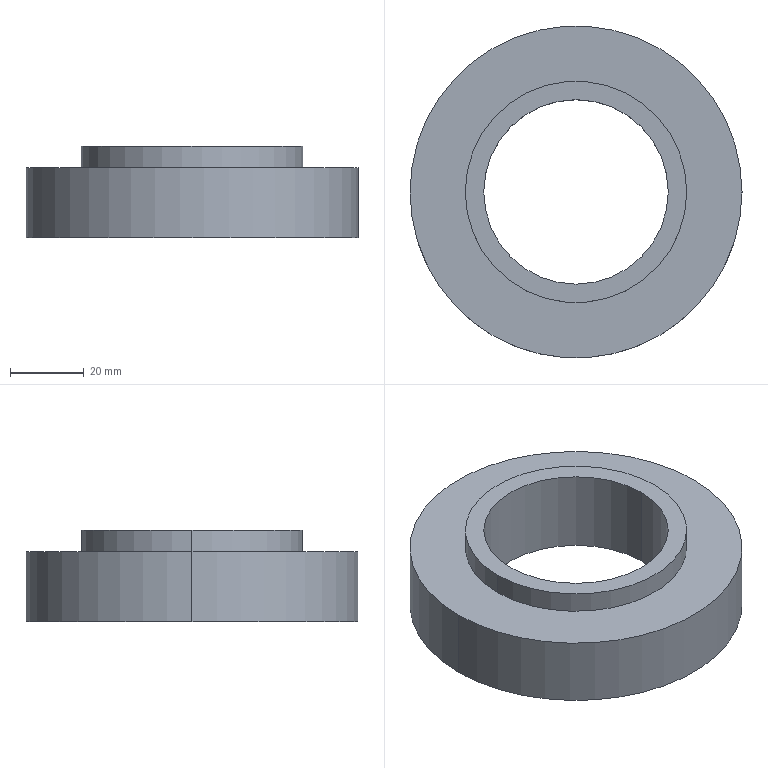Part | STEP file | 32210 | 1 solid | 12 faces | box 90 x 90 x 24.75 mm | volume 82408 mm3 | cylinder 8 | plane 4 | commonest cylinder face diameters 50 x2 60 x2 80 x2 90 x2
STEP:
#1=CARTESIAN_POINT('',(0.,0.,0.));
#2=DIRECTION('',(0.,0.,1.));
#3=DIRECTION('',(1.,0.,0.));
#4=AXIS2_PLACEMENT_3D('',#1,#2,#3);
#5=CARTESIAN_POINT('',(-40.,0.,2.));
#6=VERTEX_POINT('',#5);
#7=CARTESIAN_POINT('',(-40.,0.,0.));
#8=VERTEX_POINT('',#7);
#9=CARTESIAN_POINT('',(-40.,0.,2.));
#10=DIRECTION('',(0.,0.,-1.));
#11=VECTOR('',#10,1.);
#12=LINE('',#9,#11);
#13=CARTESIAN_POINT('',(0.,0.,2.));
#14=DIRECTION('',(0.,0.,-1.));
#15=DIRECTION('',(-1.,0.,0.));
#16=AXIS2_PLACEMENT_3D('',#13,#14,#15);
#17=CYLINDRICAL_SURFACE('',#16,40.);
#18=CARTESIAN_POINT('',(6.283,0.));
#19=DIRECTION('',(0.,1.));
#20=VECTOR('',#19,1.);
#21=LINE('',#18,#20);
#22=(GEOMETRIC_REPRESENTATION_CONTEXT(2)PARAMETRIC_REPRESENTATION_CONTEXT()REPRESENTATION_CONTEXT('',''));
#23=DEFINITIONAL_REPRESENTATION('',(#21),#22);
#24=PCURVE('',#17,#23);
#25=CARTESIAN_POINT('',(0.,0.,2.));
#26=DIRECTION('',(0.,0.,-1.));
#27=DIRECTION('',(-1.,0.,0.));
#28=AXIS2_PLACEMENT_3D('',#25,#26,#27);
#29=CYLINDRICAL_SURFACE('',#28,40.);
#30=CARTESIAN_POINT('',(0.,0.));
#31=DIRECTION('',(0.,1.));
#32=VECTOR('',#31,1.);
#33=LINE('',#30,#32);
#34=(GEOMETRIC_REPRESENTATION_CONTEXT(2)PARAMETRIC_REPRESENTATION_CONTEXT()REPRESENTATION_CONTEXT('',''));
#35=DEFINITIONAL_REPRESENTATION('',(#33),#34);
#36=PCURVE('',#29,#35);
#37=SURFACE_CURVE('',#12,(#24,#36),.PCURVE_S1.);
#38=EDGE_CURVE('',#6,#8,#37,.T.);
#39=ORIENTED_EDGE('',*,*,#38,.T.);
#40=CARTESIAN_POINT('',(40.,0.,0.));
#41=VERTEX_POINT('',#40);
#42=CARTESIAN_POINT('',(0.,0.,0.));
#43=DIRECTION('',(0.,0.,-1.));
#44=DIRECTION('',(-1.,0.,0.));
#45=AXIS2_PLACEMENT_3D('',#42,#43,#44);
#46=CIRCLE('',#45,40.);
#47=CARTESIAN_POINT('',(0.,2.));
#48=DIRECTION('',(1.,0.));
#49=VECTOR('',#48,1.);
#50=LINE('',#47,#49);
#51=(GEOMETRIC_REPRESENTATION_CONTEXT(2)PARAMETRIC_REPRESENTATION_CONTEXT()REPRESENTATION_CONTEXT('',''));
#52=DEFINITIONAL_REPRESENTATION('',(#50),#51);
#53=PCURVE('',#17,#52);
#54=CARTESIAN_POINT('',(0.,0.,0.));
#55=DIRECTION('',(0.,0.,1.));
#56=DIRECTION('',(1.,0.,0.));
#57=AXIS2_PLACEMENT_3D('',#54,#55,#56);
#58=PLANE('',#57);
#59=CARTESIAN_POINT('',(-40.,0.));
#60=CARTESIAN_POINT('',(-40.,69.282));
#61=CARTESIAN_POINT('',(20.,34.641));
#62=CARTESIAN_POINT('',(80.,0.));
#63=CARTESIAN_POINT('',(20.,-34.641));
#64=CARTESIAN_POINT('',(-40.,-69.282));
#65=CARTESIAN_POINT('',(-40.,0.));
#66=(BOUNDED_CURVE()B_SPLINE_CURVE(2,(#59,#60,#61,#62,#63,#64,#65),.UNSPECIFIED.,.T.,.F.)B_SPLINE_CURVE_WITH_KNOTS((1,2,2,2,2,1),(-2.094,0.,2.094,4.189,6.283,8.378),.UNSPECIFIED.)CURVE()GEOMETRIC_REPRESENTATION_ITEM()RATIONAL_B_SPLINE_CURVE((1.,0.5,1.,0.5,1.,0.5,1.))REPRESENTATION_ITEM(''));
#67=(GEOMETRIC_REPRESENTATION_CONTEXT(2)PARAMETRIC_REPRESENTATION_CONTEXT()REPRESENTATION_CONTEXT('',''));
#68=DEFINITIONAL_REPRESENTATION('',(#66),#67);
#69=PCURVE('',#58,#68);
#70=SURFACE_CURVE('',#46,(#53,#69),.PCURVE_S1.);
#71=EDGE_CURVE('',#41,#8,#70,.T.);
#72=ORIENTED_EDGE('',*,*,#71,.F.);
#73=CARTESIAN_POINT('',(40.,0.,2.));
#74=VERTEX_POINT('',#73);
#75=CARTESIAN_POINT('',(40.,0.,2.));
#76=DIRECTION('',(0.,0.,-1.));
#77=VECTOR('',#76,1.);
#78=LINE('',#75,#77);
#79=CARTESIAN_POINT('',(3.142,0.));
#80=DIRECTION('',(0.,1.));
#81=VECTOR('',#80,1.);
#82=LINE('',#79,#81);
#83=(GEOMETRIC_REPRESENTATION_CONTEXT(2)PARAMETRIC_REPRESENTATION_CONTEXT()REPRESENTATION_CONTEXT('',''));
#84=DEFINITIONAL_REPRESENTATION('',(#82),#83);
#85=PCURVE('',#17,#84);
#86=CARTESIAN_POINT('',(3.142,0.));
#87=DIRECTION('',(0.,1.));
#88=VECTOR('',#87,1.);
#89=LINE('',#86,#88);
#90=(GEOMETRIC_REPRESENTATION_CONTEXT(2)PARAMETRIC_REPRESENTATION_CONTEXT()REPRESENTATION_CONTEXT('',''));
#91=DEFINITIONAL_REPRESENTATION('',(#89),#90);
#92=PCURVE('',#29,#91);
#93=SURFACE_CURVE('',#78,(#85,#92),.PCURVE_S1.);
#94=EDGE_CURVE('',#74,#41,#93,.T.);
#95=ORIENTED_EDGE('',*,*,#94,.F.);
#96=CARTESIAN_POINT('',(0.,0.,2.));
#97=DIRECTION('',(0.,0.,-1.));
#98=DIRECTION('',(-1.,0.,0.));
#99=AXIS2_PLACEMENT_3D('',#96,#97,#98);
#100=CIRCLE('',#99,40.);
#101=CARTESIAN_POINT('',(0.,0.));
#102=DIRECTION('',(1.,0.));
#103=VECTOR('',#102,1.);
#104=LINE('',#101,#103);
#105=(GEOMETRIC_REPRESENTATION_CONTEXT(2)PARAMETRIC_REPRESENTATION_CONTEXT()REPRESENTATION_CONTEXT('',''));
#106=DEFINITIONAL_REPRESENTATION('',(#104),#105);
#107=PCURVE('',#17,#106);
#108=CARTESIAN_POINT('',(0.,0.,2.));
#109=DIRECTION('',(0.,0.,-1.));
#110=DIRECTION('',(-1.,0.,0.));
#111=AXIS2_PLACEMENT_3D('',#108,#109,#110);
#112=PLANE('',#111);
#113=CARTESIAN_POINT('',(0.,0.));
#114=DIRECTION('',(1.,0.));
#115=AXIS2_PLACEMENT_2D('',#113,#114);
#116=CIRCLE('',#115,40.);
#117=(GEOMETRIC_REPRESENTATION_CONTEXT(2)PARAMETRIC_REPRESENTATION_CONTEXT()REPRESENTATION_CONTEXT('',''));
#118=DEFINITIONAL_REPRESENTATION('',(#116),#117);
#119=PCURVE('',#112,#118);
#120=SURFACE_CURVE('',#100,(#107,#119),.PCURVE_S1.);
#121=EDGE_CURVE('',#74,#6,#120,.T.);
#122=ORIENTED_EDGE('',*,*,#121,.T.);
#123=EDGE_LOOP('',(#39,#72,#95,#122));
#124=FACE_BOUND('',#123,.F.);
#125=ADVANCED_FACE('',(#124),#17,.F.);
#126=CARTESIAN_POINT('',(30.,0.,19.));
#127=VERTEX_POINT('',#126);
#128=CARTESIAN_POINT('',(-30.,0.,19.));
#129=VERTEX_POINT('',#128);
#130=CARTESIAN_POINT('',(0.,0.,19.));
#131=DIRECTION('',(0.,0.,1.));
#132=DIRECTION('',(1.,0.,0.));
#133=AXIS2_PLACEMENT_3D('',#130,#131,#132);
#134=CIRCLE('',#133,30.);
#135=CARTESIAN_POINT('',(0.,0.,19.));
#136=DIRECTION('',(0.,0.,1.));
#137=DIRECTION('',(1.,0.,0.));
#138=AXIS2_PLACEMENT_3D('',#135,#136,#137);
#139=CYLINDRICAL_SURFACE('',#138,30.);
#140=CARTESIAN_POINT('',(0.,0.));
#141=DIRECTION('',(1.,0.));
#142=VECTOR('',#141,1.);
#143=LINE('',#140,#142);
#144=(GEOMETRIC_REPRESENTATION_CONTEXT(2)PARAMETRIC_REPRESENTATION_CONTEXT()REPRESENTATION_CONTEXT('',''));
#145=DEFINITIONAL_REPRESENTATION('',(#143),#144);
#146=PCURVE('',#139,#145);
#147=CARTESIAN_POINT('',(0.,0.,19.));
#148=DIRECTION('',(0.,0.,1.));
#149=DIRECTION('',(1.,0.,0.));
#150=AXIS2_PLACEMENT_3D('',#147,#148,#149);
#151=PLANE('',#150);
#152=CARTESIAN_POINT('',(0.,0.));
#153=DIRECTION('',(1.,0.));
#154=AXIS2_PLACEMENT_2D('',#152,#153);
#155=CIRCLE('',#154,30.);
#156=(GEOMETRIC_REPRESENTATION_CONTEXT(2)PARAMETRIC_REPRESENTATION_CONTEXT()REPRESENTATION_CONTEXT('',''));
#157=DEFINITIONAL_REPRESENTATION('',(#155),#156);
#158=PCURVE('',#151,#157);
#159=SURFACE_CURVE('',#134,(#146,#158),.PCURVE_S1.);
#160=EDGE_CURVE('',#127,#129,#159,.T.);
#161=ORIENTED_EDGE('',*,*,#160,.T.);
#162=CARTESIAN_POINT('',(-30.,0.,24.75));
#163=VERTEX_POINT('',#162);
#164=CARTESIAN_POINT('',(-30.,0.,19.));
#165=DIRECTION('',(0.,0.,1.));
#166=VECTOR('',#165,1.);
#167=LINE('',#164,#166);
#168=CARTESIAN_POINT('',(3.142,0.));
#169=DIRECTION('',(0.,1.));
#170=VECTOR('',#169,1.);
#171=LINE('',#168,#170);
#172=(GEOMETRIC_REPRESENTATION_CONTEXT(2)PARAMETRIC_REPRESENTATION_CONTEXT()REPRESENTATION_CONTEXT('',''));
#173=DEFINITIONAL_REPRESENTATION('',(#171),#172);
#174=PCURVE('',#139,#173);
#175=CARTESIAN_POINT('',(0.,0.,19.));
#176=DIRECTION('',(0.,0.,1.));
#177=DIRECTION('',(1.,0.,0.));
#178=AXIS2_PLACEMENT_3D('',#175,#176,#177);
#179=CYLINDRICAL_SURFACE('',#178,30.);
#180=CARTESIAN_POINT('',(3.142,0.));
#181=DIRECTION('',(0.,1.));
#182=VECTOR('',#181,1.);
#183=LINE('',#180,#182);
#184=(GEOMETRIC_REPRESENTATION_CONTEXT(2)PARAMETRIC_REPRESENTATION_CONTEXT()REPRESENTATION_CONTEXT('',''));
#185=DEFINITIONAL_REPRESENTATION('',(#183),#184);
#186=PCURVE('',#179,#185);
#187=SURFACE_CURVE('',#167,(#174,#186),.PCURVE_S1.);
#188=EDGE_CURVE('',#129,#163,#187,.T.);
#189=ORIENTED_EDGE('',*,*,#188,.T.);
#190=CARTESIAN_POINT('',(30.,0.,24.75));
#191=VERTEX_POINT('',#190);
#192=CARTESIAN_POINT('',(0.,0.,24.75));
#193=DIRECTION('',(0.,0.,1.));
#194=DIRECTION('',(1.,0.,0.));
#195=AXIS2_PLACEMENT_3D('',#192,#193,#194);
#196=CIRCLE('',#195,30.);
#197=CARTESIAN_POINT('',(0.,5.75));
#198=DIRECTION('',(1.,0.));
#199=VECTOR('',#198,1.);
#200=LINE('',#197,#199);
#201=(GEOMETRIC_REPRESENTATION_CONTEXT(2)PARAMETRIC_REPRESENTATION_CONTEXT()REPRESENTATION_CONTEXT('',''));
#202=DEFINITIONAL_REPRESENTATION('',(#200),#201);
#203=PCURVE('',#139,#202);
#204=CARTESIAN_POINT('',(0.,0.,24.75));
#205=DIRECTION('',(0.,0.,1.));
#206=DIRECTION('',(1.,0.,0.));
#207=AXIS2_PLACEMENT_3D('',#204,#205,#206);
#208=PLANE('',#207);
#209=CARTESIAN_POINT('',(0.,0.));
#210=DIRECTION('',(1.,0.));
#211=AXIS2_PLACEMENT_2D('',#209,#210);
#212=CIRCLE('',#211,30.);
#213=(GEOMETRIC_REPRESENTATION_CONTEXT(2)PARAMETRIC_REPRESENTATION_CONTEXT()REPRESENTATION_CONTEXT('',''));
#214=DEFINITIONAL_REPRESENTATION('',(#212),#213);
#215=PCURVE('',#208,#214);
#216=SURFACE_CURVE('',#196,(#203,#215),.PCURVE_S1.);
#217=EDGE_CURVE('',#191,#163,#216,.T.);
#218=ORIENTED_EDGE('',*,*,#217,.F.);
#219=CARTESIAN_POINT('',(30.,0.,19.));
#220=DIRECTION('',(0.,0.,1.));
#221=VECTOR('',#220,1.);
#222=LINE('',#219,#221);
#223=CARTESIAN_POINT('',(0.,0.));
#224=DIRECTION('',(0.,1.));
#225=VECTOR('',#224,1.);
#226=LINE('',#223,#225);
#227=(GEOMETRIC_REPRESENTATION_CONTEXT(2)PARAMETRIC_REPRESENTATION_CONTEXT()REPRESENTATION_CONTEXT('',''));
#228=DEFINITIONAL_REPRESENTATION('',(#226),#227);
#229=PCURVE('',#139,#228);
#230=CARTESIAN_POINT('',(6.283,0.));
#231=DIRECTION('',(0.,1.));
#232=VECTOR('',#231,1.);
#233=LINE('',#230,#232);
#234=(GEOMETRIC_REPRESENTATION_CONTEXT(2)PARAMETRIC_REPRESENTATION_CONTEXT()REPRESENTATION_CONTEXT('',''));
#235=DEFINITIONAL_REPRESENTATION('',(#233),#234);
#236=PCURVE('',#179,#235);
#237=SURFACE_CURVE('',#222,(#229,#236),.PCURVE_S1.);
#238=EDGE_CURVE('',#127,#191,#237,.T.);
#239=ORIENTED_EDGE('',*,*,#238,.F.);
#240=EDGE_LOOP('',(#161,#189,#218,#239));
#241=FACE_BOUND('',#240,.T.);
#242=ADVANCED_FACE('',(#241),#139,.T.);
#243=CARTESIAN_POINT('',(45.,0.,19.));
#244=VERTEX_POINT('',#243);
#245=CARTESIAN_POINT('',(-45.,0.,19.));
#246=VERTEX_POINT('',#245);
#247=CARTESIAN_POINT('',(0.,0.,19.));
#248=DIRECTION('',(0.,0.,1.));
#249=DIRECTION('',(1.,0.,0.));
#250=AXIS2_PLACEMENT_3D('',#247,#248,#249);
#251=CIRCLE('',#250,45.);
#252=CARTESIAN_POINT('',(0.,0.,24.75));
#253=DIRECTION('',(0.,0.,-1.));
#254=DIRECTION('',(-1.,0.,0.));
#255=AXIS2_PLACEMENT_3D('',#252,#253,#254);
#256=CYLINDRICAL_SURFACE('',#255,45.);
#257=CARTESIAN_POINT('',(3.142,5.75));
#258=DIRECTION('',(-1.,0.));
#259=VECTOR('',#258,1.);
#260=LINE('',#257,#259);
#261=(GEOMETRIC_REPRESENTATION_CONTEXT(2)PARAMETRIC_REPRESENTATION_CONTEXT()REPRESENTATION_CONTEXT('',''));
#262=DEFINITIONAL_REPRESENTATION('',(#260),#261);
#263=PCURVE('',#256,#262);
#264=CARTESIAN_POINT('',(0.,0.));
#265=DIRECTION('',(1.,0.));
#266=AXIS2_PLACEMENT_2D('',#264,#265);
#267=CIRCLE('',#266,45.);
#268=(GEOMETRIC_REPRESENTATION_CONTEXT(2)PARAMETRIC_REPRESENTATION_CONTEXT()REPRESENTATION_CONTEXT('',''));
#269=DEFINITIONAL_REPRESENTATION('',(#267),#268);
#270=PCURVE('',#151,#269);
#271=SURFACE_CURVE('',#251,(#263,#270),.PCURVE_S1.);
#272=EDGE_CURVE('',#244,#246,#271,.T.);
#273=ORIENTED_EDGE('',*,*,#272,.F.);
#274=CARTESIAN_POINT('',(45.,0.,0.));
#275=VERTEX_POINT('',#274);
#276=CARTESIAN_POINT('',(45.,0.,24.75));
#277=DIRECTION('',(0.,0.,-1.));
#278=VECTOR('',#277,1.);
#279=LINE('',#276,#278);
#280=CARTESIAN_POINT('',(3.142,0.));
#281=DIRECTION('',(0.,1.));
#282=VECTOR('',#281,1.);
#283=LINE('',#280,#282);
#284=(GEOMETRIC_REPRESENTATION_CONTEXT(2)PARAMETRIC_REPRESENTATION_CONTEXT()REPRESENTATION_CONTEXT('',''));
#285=DEFINITIONAL_REPRESENTATION('',(#283),#284);
#286=PCURVE('',#256,#285);
#287=CARTESIAN_POINT('',(0.,0.,24.75));
#288=DIRECTION('',(0.,0.,-1.));
#289=DIRECTION('',(-1.,0.,0.));
#290=AXIS2_PLACEMENT_3D('',#287,#288,#289);
#291=CYLINDRICAL_SURFACE('',#290,45.);
#292=CARTESIAN_POINT('',(3.142,0.));
#293=DIRECTION('',(0.,1.));
#294=VECTOR('',#293,1.);
#295=LINE('',#292,#294);
#296=(GEOMETRIC_REPRESENTATION_CONTEXT(2)PARAMETRIC_REPRESENTATION_CONTEXT()REPRESENTATION_CONTEXT('',''));
#297=DEFINITIONAL_REPRESENTATION('',(#295),#296);
#298=PCURVE('',#291,#297);
#299=SURFACE_CURVE('',#279,(#286,#298),.PCURVE_S1.);
#300=EDGE_CURVE('',#244,#275,#299,.T.);
#301=ORIENTED_EDGE('',*,*,#300,.T.);
#302=CARTESIAN_POINT('',(-45.,0.,0.));
#303=VERTEX_POINT('',#302);
#304=CARTESIAN_POINT('',(0.,0.,0.));
#305=DIRECTION('',(0.,0.,1.));
#306=DIRECTION('',(1.,0.,0.));
#307=AXIS2_PLACEMENT_3D('',#304,#305,#306);
#308=CIRCLE('',#307,45.);
#309=CARTESIAN_POINT('',(3.142,24.75));
#310=DIRECTION('',(-1.,0.));
#311=VECTOR('',#310,1.);
#312=LINE('',#309,#311);
#313=(GEOMETRIC_REPRESENTATION_CONTEXT(2)PARAMETRIC_REPRESENTATION_CONTEXT()REPRESENTATION_CONTEXT('',''));
#314=DEFINITIONAL_REPRESENTATION('',(#312),#313);
#315=PCURVE('',#256,#314);
#316=CARTESIAN_POINT('',(0.,0.));
#317=DIRECTION('',(1.,0.));
#318=AXIS2_PLACEMENT_2D('',#316,#317);
#319=CIRCLE('',#318,45.);
#320=(GEOMETRIC_REPRESENTATION_CONTEXT(2)PARAMETRIC_REPRESENTATION_CONTEXT()REPRESENTATION_CONTEXT('',''));
#321=DEFINITIONAL_REPRESENTATION('',(#319),#320);
#322=PCURVE('',#58,#321);
#323=SURFACE_CURVE('',#308,(#315,#322),.PCURVE_S1.);
#324=EDGE_CURVE('',#275,#303,#323,.T.);
#325=ORIENTED_EDGE('',*,*,#324,.T.);
#326=CARTESIAN_POINT('',(-45.,0.,24.75));
#327=DIRECTION('',(0.,0.,-1.));
#328=VECTOR('',#327,1.);
#329=LINE('',#326,#328);
#330=CARTESIAN_POINT('',(0.,0.));
#331=DIRECTION('',(0.,1.));
#332=VECTOR('',#331,1.);
#333=LINE('',#330,#332);
#334=(GEOMETRIC_REPRESENTATION_CONTEXT(2)PARAMETRIC_REPRESENTATION_CONTEXT()REPRESENTATION_CONTEXT('',''));
#335=DEFINITIONAL_REPRESENTATION('',(#333),#334);
#336=PCURVE('',#256,#335);
#337=CARTESIAN_POINT('',(6.283,0.));
#338=DIRECTION('',(0.,1.));
#339=VECTOR('',#338,1.);
#340=LINE('',#337,#339);
#341=(GEOMETRIC_REPRESENTATION_CONTEXT(2)PARAMETRIC_REPRESENTATION_CONTEXT()REPRESENTATION_CONTEXT('',''));
#342=DEFINITIONAL_REPRESENTATION('',(#340),#341);
#343=PCURVE('',#291,#342);
#344=SURFACE_CURVE('',#329,(#336,#343),.PCURVE_S1.);
#345=EDGE_CURVE('',#246,#303,#344,.T.);
#346=ORIENTED_EDGE('',*,*,#345,.F.);
#347=EDGE_LOOP('',(#273,#301,#325,#346));
#348=FACE_BOUND('',#347,.T.);
#349=ADVANCED_FACE('',(#348),#256,.T.);
#350=CARTESIAN_POINT('',(-25.,0.,24.75));
#351=VERTEX_POINT('',#350);
#352=CARTESIAN_POINT('',(-25.,0.,2.));
#353=VERTEX_POINT('',#352);
#354=CARTESIAN_POINT('',(-25.,0.,24.75));
#355=DIRECTION('',(0.,0.,-1.));
#356=VECTOR('',#355,1.);
#357=LINE('',#354,#356);
#358=CARTESIAN_POINT('',(0.,0.,24.75));
#359=DIRECTION('',(0.,0.,-1.));
#360=DIRECTION('',(-1.,0.,0.));
#361=AXIS2_PLACEMENT_3D('',#358,#359,#360);
#362=CYLINDRICAL_SURFACE('',#361,25.);
#363=CARTESIAN_POINT('',(6.283,0.));
#364=DIRECTION('',(0.,1.));
#365=VECTOR('',#364,1.);
#366=LINE('',#363,#365);
#367=(GEOMETRIC_REPRESENTATION_CONTEXT(2)PARAMETRIC_REPRESENTATION_CONTEXT()REPRESENTATION_CONTEXT('',''));
#368=DEFINITIONAL_REPRESENTATION('',(#366),#367);
#369=PCURVE('',#362,#368);
#370=CARTESIAN_POINT('',(0.,0.,24.75));
#371=DIRECTION('',(0.,0.,-1.));
#372=DIRECTION('',(-1.,0.,0.));
#373=AXIS2_PLACEMENT_3D('',#370,#371,#372);
#374=CYLINDRICAL_SURFACE('',#373,25.);
#375=CARTESIAN_POINT('',(0.,0.));
#376=DIRECTION('',(0.,1.));
#377=VECTOR('',#376,1.);
#378=LINE('',#375,#377);
#379=(GEOMETRIC_REPRESENTATION_CONTEXT(2)PARAMETRIC_REPRESENTATION_CONTEXT()REPRESENTATION_CONTEXT('',''));
#380=DEFINITIONAL_REPRESENTATION('',(#378),#379);
#381=PCURVE('',#374,#380);
#382=SURFACE_CURVE('',#357,(#369,#381),.PCURVE_S1.);
#383=EDGE_CURVE('',#351,#353,#382,.T.);
#384=ORIENTED_EDGE('',*,*,#383,.T.);
#385=CARTESIAN_POINT('',(25.,0.,2.));
#386=VERTEX_POINT('',#385);
#387=CARTESIAN_POINT('',(0.,0.,2.));
#388=DIRECTION('',(0.,0.,-1.));
#389=DIRECTION('',(-1.,0.,0.));
#390=AXIS2_PLACEMENT_3D('',#387,#388,#389);
#391=CIRCLE('',#390,25.);
#392=CARTESIAN_POINT('',(0.,22.75));
#393=DIRECTION('',(1.,0.));
#394=VECTOR('',#393,1.);
#395=LINE('',#392,#394);
#396=(GEOMETRIC_REPRESENTATION_CONTEXT(2)PARAMETRIC_REPRESENTATION_CONTEXT()REPRESENTATION_CONTEXT('',''));
#397=DEFINITIONAL_REPRESENTATION('',(#395),#396);
#398=PCURVE('',#362,#397);
#399=CARTESIAN_POINT('',(0.,0.));
#400=DIRECTION('',(1.,0.));
#401=AXIS2_PLACEMENT_2D('',#399,#400);
#402=CIRCLE('',#401,25.);
#403=(GEOMETRIC_REPRESENTATION_CONTEXT(2)PARAMETRIC_REPRESENTATION_CONTEXT()REPRESENTATION_CONTEXT('',''));
#404=DEFINITIONAL_REPRESENTATION('',(#402),#403);
#405=PCURVE('',#112,#404);
#406=SURFACE_CURVE('',#391,(#398,#405),.PCURVE_S1.);
#407=EDGE_CURVE('',#386,#353,#406,.T.);
#408=ORIENTED_EDGE('',*,*,#407,.F.);
#409=CARTESIAN_POINT('',(25.,0.,24.75));
#410=VERTEX_POINT('',#409);
#411=CARTESIAN_POINT('',(25.,0.,24.75));
#412=DIRECTION('',(0.,0.,-1.));
#413=VECTOR('',#412,1.);
#414=LINE('',#411,#413);
#415=CARTESIAN_POINT('',(3.142,0.));
#416=DIRECTION('',(0.,1.));
#417=VECTOR('',#416,1.);
#418=LINE('',#415,#417);
#419=(GEOMETRIC_REPRESENTATION_CONTEXT(2)PARAMETRIC_REPRESENTATION_CONTEXT()REPRESENTATION_CONTEXT('',''));
#420=DEFINITIONAL_REPRESENTATION('',(#418),#419);
#421=PCURVE('',#362,#420);
#422=CARTESIAN_POINT('',(3.142,0.));
#423=DIRECTION('',(0.,1.));
#424=VECTOR('',#423,1.);
#425=LINE('',#422,#424);
#426=(GEOMETRIC_REPRESENTATION_CONTEXT(2)PARAMETRIC_REPRESENTATION_CONTEXT()REPRESENTATION_CONTEXT('',''));
#427=DEFINITIONAL_REPRESENTATION('',(#425),#426);
#428=PCURVE('',#374,#427);
#429=SURFACE_CURVE('',#414,(#421,#428),.PCURVE_S1.);
#430=EDGE_CURVE('',#410,#386,#429,.T.);
#431=ORIENTED_EDGE('',*,*,#430,.F.);
#432=CARTESIAN_POINT('',(0.,0.,24.75));
#433=DIRECTION('',(0.,0.,1.));
#434=DIRECTION('',(1.,0.,0.));
#435=AXIS2_PLACEMENT_3D('',#432,#433,#434);
#436=CIRCLE('',#435,25.);
#437=CARTESIAN_POINT('',(9.425,0.));
#438=DIRECTION('',(-1.,0.));
#439=VECTOR('',#438,1.);
#440=LINE('',#437,#439);
#441=(GEOMETRIC_REPRESENTATION_CONTEXT(2)PARAMETRIC_REPRESENTATION_CONTEXT()REPRESENTATION_CONTEXT('',''));
#442=DEFINITIONAL_REPRESENTATION('',(#440),#441);
#443=PCURVE('',#362,#442);
#444=CARTESIAN_POINT('',(0.,0.));
#445=DIRECTION('',(1.,0.));
#446=AXIS2_PLACEMENT_2D('',#444,#445);
#447=CIRCLE('',#446,25.);
#448=(GEOMETRIC_REPRESENTATION_CONTEXT(2)PARAMETRIC_REPRESENTATION_CONTEXT()REPRESENTATION_CONTEXT('',''));
#449=DEFINITIONAL_REPRESENTATION('',(#447),#448);
#450=PCURVE('',#208,#449);
#451=SURFACE_CURVE('',#436,(#443,#450),.PCURVE_S1.);
#452=EDGE_CURVE('',#351,#410,#451,.T.);
#453=ORIENTED_EDGE('',*,*,#452,.F.);
#454=EDGE_LOOP('',(#384,#408,#431,#453));
#455=FACE_BOUND('',#454,.F.);
#456=ADVANCED_FACE('',(#455),#362,.F.);
#457=CARTESIAN_POINT('',(0.,0.,2.));
#458=DIRECTION('',(0.,0.,-1.));
#459=DIRECTION('',(-1.,0.,0.));
#460=AXIS2_PLACEMENT_3D('',#457,#458,#459);
#461=CIRCLE('',#460,25.);
#462=CARTESIAN_POINT('',(0.,22.75));
#463=DIRECTION('',(1.,0.));
#464=VECTOR('',#463,1.);
#465=LINE('',#462,#464);
#466=(GEOMETRIC_REPRESENTATION_CONTEXT(2)PARAMETRIC_REPRESENTATION_CONTEXT()REPRESENTATION_CONTEXT('',''));
#467=DEFINITIONAL_REPRESENTATION('',(#465),#466);
#468=PCURVE('',#374,#467);
#469=CARTESIAN_POINT('',(0.,0.));
#470=DIRECTION('',(1.,0.));
#471=AXIS2_PLACEMENT_2D('',#469,#470);
#472=CIRCLE('',#471,25.);
#473=(GEOMETRIC_REPRESENTATION_CONTEXT(2)PARAMETRIC_REPRESENTATION_CONTEXT()REPRESENTATION_CONTEXT('',''));
#474=DEFINITIONAL_REPRESENTATION('',(#472),#473);
#475=PCURVE('',#112,#474);
#476=SURFACE_CURVE('',#461,(#468,#475),.PCURVE_S1.);
#477=EDGE_CURVE('',#353,#386,#476,.T.);
#478=ORIENTED_EDGE('',*,*,#477,.F.);
#479=ORIENTED_EDGE('',*,*,#383,.F.);
#480=CARTESIAN_POINT('',(0.,0.,24.75));
#481=DIRECTION('',(0.,0.,1.));
#482=DIRECTION('',(1.,0.,0.));
#483=AXIS2_PLACEMENT_3D('',#480,#481,#482);
#484=CIRCLE('',#483,25.);
#485=CARTESIAN_POINT('',(3.142,0.));
#486=DIRECTION('',(-1.,0.));
#487=VECTOR('',#486,1.);
#488=LINE('',#485,#487);
#489=(GEOMETRIC_REPRESENTATION_CONTEXT(2)PARAMETRIC_REPRESENTATION_CONTEXT()REPRESENTATION_CONTEXT('',''));
#490=DEFINITIONAL_REPRESENTATION('',(#488),#489);
#491=PCURVE('',#374,#490);
#492=CARTESIAN_POINT('',(0.,0.));
#493=DIRECTION('',(1.,0.));
#494=AXIS2_PLACEMENT_2D('',#492,#493);
#495=CIRCLE('',#494,25.);
#496=(GEOMETRIC_REPRESENTATION_CONTEXT(2)PARAMETRIC_REPRESENTATION_CONTEXT()REPRESENTATION_CONTEXT('',''));
#497=DEFINITIONAL_REPRESENTATION('',(#495),#496);
#498=PCURVE('',#208,#497);
#499=SURFACE_CURVE('',#484,(#491,#498),.PCURVE_S1.);
#500=EDGE_CURVE('',#410,#351,#499,.T.);
#501=ORIENTED_EDGE('',*,*,#500,.F.);
#502=ORIENTED_EDGE('',*,*,#430,.T.);
#503=EDGE_LOOP('',(#478,#479,#501,#502));
#504=FACE_BOUND('',#503,.F.);
#505=ADVANCED_FACE('',(#504),#374,.F.);
#506=ORIENTED_EDGE('',*,*,#452,.F.);
#507=ORIENTED_EDGE('',*,*,#500,.F.);
#508=EDGE_LOOP('',(#506,#507));
#509=FACE_BOUND('',#508,.T.);
#510=ORIENTED_EDGE('',*,*,#217,.T.);
#511=CARTESIAN_POINT('',(0.,0.,24.75));
#512=DIRECTION('',(0.,0.,1.));
#513=DIRECTION('',(1.,0.,0.));
#514=AXIS2_PLACEMENT_3D('',#511,#512,#513);
#515=CIRCLE('',#514,30.);
#516=CARTESIAN_POINT('',(0.,0.));
#517=DIRECTION('',(1.,0.));
#518=AXIS2_PLACEMENT_2D('',#516,#517);
#519=CIRCLE('',#518,30.);
#520=(GEOMETRIC_REPRESENTATION_CONTEXT(2)PARAMETRIC_REPRESENTATION_CONTEXT()REPRESENTATION_CONTEXT('',''));
#521=DEFINITIONAL_REPRESENTATION('',(#519),#520);
#522=PCURVE('',#208,#521);
#523=CARTESIAN_POINT('',(0.,5.75));
#524=DIRECTION('',(1.,0.));
#525=VECTOR('',#524,1.);
#526=LINE('',#523,#525);
#527=(GEOMETRIC_REPRESENTATION_CONTEXT(2)PARAMETRIC_REPRESENTATION_CONTEXT()REPRESENTATION_CONTEXT('',''));
#528=DEFINITIONAL_REPRESENTATION('',(#526),#527);
#529=PCURVE('',#179,#528);
#530=SURFACE_CURVE('',#515,(#522,#529),.PCURVE_S1.);
#531=EDGE_CURVE('',#163,#191,#530,.T.);
#532=ORIENTED_EDGE('',*,*,#531,.T.);
#533=EDGE_LOOP('',(#510,#532));
#534=FACE_BOUND('',#533,.T.);
#535=ADVANCED_FACE('',(#509,#534),#208,.T.);
#536=ORIENTED_EDGE('',*,*,#300,.F.);
#537=CARTESIAN_POINT('',(0.,0.,19.));
#538=DIRECTION('',(0.,0.,1.));
#539=DIRECTION('',(1.,0.,0.));
#540=AXIS2_PLACEMENT_3D('',#537,#538,#539);
#541=CIRCLE('',#540,45.);
#542=CARTESIAN_POINT('',(9.425,5.75));
#543=DIRECTION('',(-1.,0.));
#544=VECTOR('',#543,1.);
#545=LINE('',#542,#544);
#546=(GEOMETRIC_REPRESENTATION_CONTEXT(2)PARAMETRIC_REPRESENTATION_CONTEXT()REPRESENTATION_CONTEXT('',''));
#547=DEFINITIONAL_REPRESENTATION('',(#545),#546);
#548=PCURVE('',#291,#547);
#549=CARTESIAN_POINT('',(0.,0.));
#550=DIRECTION('',(1.,0.));
#551=AXIS2_PLACEMENT_2D('',#549,#550);
#552=CIRCLE('',#551,45.);
#553=(GEOMETRIC_REPRESENTATION_CONTEXT(2)PARAMETRIC_REPRESENTATION_CONTEXT()REPRESENTATION_CONTEXT('',''));
#554=DEFINITIONAL_REPRESENTATION('',(#552),#553);
#555=PCURVE('',#151,#554);
#556=SURFACE_CURVE('',#541,(#548,#555),.PCURVE_S1.);
#557=EDGE_CURVE('',#246,#244,#556,.T.);
#558=ORIENTED_EDGE('',*,*,#557,.F.);
#559=ORIENTED_EDGE('',*,*,#345,.T.);
#560=CARTESIAN_POINT('',(0.,0.,0.));
#561=DIRECTION('',(0.,0.,1.));
#562=DIRECTION('',(1.,0.,0.));
#563=AXIS2_PLACEMENT_3D('',#560,#561,#562);
#564=CIRCLE('',#563,45.);
#565=CARTESIAN_POINT('',(9.425,24.75));
#566=DIRECTION('',(-1.,0.));
#567=VECTOR('',#566,1.);
#568=LINE('',#565,#567);
#569=(GEOMETRIC_REPRESENTATION_CONTEXT(2)PARAMETRIC_REPRESENTATION_CONTEXT()REPRESENTATION_CONTEXT('',''));
#570=DEFINITIONAL_REPRESENTATION('',(#568),#569);
#571=PCURVE('',#291,#570);
#572=CARTESIAN_POINT('',(0.,0.));
#573=DIRECTION('',(1.,0.));
#574=AXIS2_PLACEMENT_2D('',#572,#573);
#575=CIRCLE('',#574,45.);
#576=(GEOMETRIC_REPRESENTATION_CONTEXT(2)PARAMETRIC_REPRESENTATION_CONTEXT()REPRESENTATION_CONTEXT('',''));
#577=DEFINITIONAL_REPRESENTATION('',(#575),#576);
#578=PCURVE('',#58,#577);
#579=SURFACE_CURVE('',#564,(#571,#578),.PCURVE_S1.);
#580=EDGE_CURVE('',#303,#275,#579,.T.);
#581=ORIENTED_EDGE('',*,*,#580,.T.);
#582=EDGE_LOOP('',(#536,#558,#559,#581));
#583=FACE_BOUND('',#582,.T.);
#584=ADVANCED_FACE('',(#583),#291,.T.);
#585=CARTESIAN_POINT('',(0.,0.,0.));
#586=DIRECTION('',(0.,0.,-1.));
#587=DIRECTION('',(-1.,0.,0.));
#588=AXIS2_PLACEMENT_3D('',#585,#586,#587);
#589=CIRCLE('',#588,40.);
#590=CARTESIAN_POINT('',(-40.,0.));
#591=CARTESIAN_POINT('',(-40.,69.282));
#592=CARTESIAN_POINT('',(20.,34.641));
#593=CARTESIAN_POINT('',(80.,0.));
#594=CARTESIAN_POINT('',(20.,-34.641));
#595=CARTESIAN_POINT('',(-40.,-69.282));
#596=CARTESIAN_POINT('',(-40.,0.));
#597=(BOUNDED_CURVE()B_SPLINE_CURVE(2,(#590,#591,#592,#593,#594,#595,#596),.UNSPECIFIED.,.T.,.F.)B_SPLINE_CURVE_WITH_KNOTS((1,2,2,2,2,1),(-2.094,0.,2.094,4.189,6.283,8.378),.UNSPECIFIED.)CURVE()GEOMETRIC_REPRESENTATION_ITEM()RATIONAL_B_SPLINE_CURVE((1.,0.5,1.,0.5,1.,0.5,1.))REPRESENTATION_ITEM(''));
#598=(GEOMETRIC_REPRESENTATION_CONTEXT(2)PARAMETRIC_REPRESENTATION_CONTEXT()REPRESENTATION_CONTEXT('',''));
#599=DEFINITIONAL_REPRESENTATION('',(#597),#598);
#600=PCURVE('',#58,#599);
#601=CARTESIAN_POINT('',(0.,2.));
#602=DIRECTION('',(1.,0.));
#603=VECTOR('',#602,1.);
#604=LINE('',#601,#603);
#605=(GEOMETRIC_REPRESENTATION_CONTEXT(2)PARAMETRIC_REPRESENTATION_CONTEXT()REPRESENTATION_CONTEXT('',''));
#606=DEFINITIONAL_REPRESENTATION('',(#604),#605);
#607=PCURVE('',#29,#606);
#608=SURFACE_CURVE('',#589,(#600,#607),.PCURVE_S1.);
#609=EDGE_CURVE('',#8,#41,#608,.T.);
#610=ORIENTED_EDGE('',*,*,#609,.F.);
#611=ORIENTED_EDGE('',*,*,#71,.F.);
#612=EDGE_LOOP('',(#610,#611));
#613=FACE_BOUND('',#612,.T.);
#614=ORIENTED_EDGE('',*,*,#580,.F.);
#615=ORIENTED_EDGE('',*,*,#324,.F.);
#616=EDGE_LOOP('',(#614,#615));
#617=FACE_BOUND('',#616,.T.);
#618=ADVANCED_FACE('',(#613,#617),#58,.F.);
#619=ORIENTED_EDGE('',*,*,#160,.F.);
#620=CARTESIAN_POINT('',(0.,0.,19.));
#621=DIRECTION('',(0.,0.,1.));
#622=DIRECTION('',(1.,0.,0.));
#623=AXIS2_PLACEMENT_3D('',#620,#621,#622);
#624=CIRCLE('',#623,30.);
#625=CARTESIAN_POINT('',(0.,0.));
#626=DIRECTION('',(1.,0.));
#627=AXIS2_PLACEMENT_2D('',#625,#626);
#628=CIRCLE('',#627,30.);
#629=(GEOMETRIC_REPRESENTATION_CONTEXT(2)PARAMETRIC_REPRESENTATION_CONTEXT()REPRESENTATION_CONTEXT('',''));
#630=DEFINITIONAL_REPRESENTATION('',(#628),#629);
#631=PCURVE('',#151,#630);
#632=CARTESIAN_POINT('',(0.,0.));
#633=DIRECTION('',(1.,0.));
#634=VECTOR('',#633,1.);
#635=LINE('',#632,#634);
#636=(GEOMETRIC_REPRESENTATION_CONTEXT(2)PARAMETRIC_REPRESENTATION_CONTEXT()REPRESENTATION_CONTEXT('',''));
#637=DEFINITIONAL_REPRESENTATION('',(#635),#636);
#638=PCURVE('',#179,#637);
#639=SURFACE_CURVE('',#624,(#631,#638),.PCURVE_S1.);
#640=EDGE_CURVE('',#129,#127,#639,.T.);
#641=ORIENTED_EDGE('',*,*,#640,.F.);
#642=EDGE_LOOP('',(#619,#641));
#643=FACE_BOUND('',#642,.T.);
#644=ORIENTED_EDGE('',*,*,#557,.T.);
#645=ORIENTED_EDGE('',*,*,#272,.T.);
#646=EDGE_LOOP('',(#644,#645));
#647=FACE_BOUND('',#646,.T.);
#648=ADVANCED_FACE('',(#643,#647),#151,.T.);
#649=ORIENTED_EDGE('',*,*,#188,.F.);
#650=ORIENTED_EDGE('',*,*,#640,.T.);
#651=ORIENTED_EDGE('',*,*,#238,.T.);
#652=ORIENTED_EDGE('',*,*,#531,.F.);
#653=EDGE_LOOP('',(#649,#650,#651,#652));
#654=FACE_BOUND('',#653,.T.);
#655=ADVANCED_FACE('',(#654),#179,.T.);
#656=ORIENTED_EDGE('',*,*,#609,.F.);
#657=ORIENTED_EDGE('',*,*,#38,.F.);
#658=CARTESIAN_POINT('',(0.,0.,2.));
#659=DIRECTION('',(0.,0.,-1.));
#660=DIRECTION('',(-1.,0.,0.));
#661=AXIS2_PLACEMENT_3D('',#658,#659,#660);
#662=CIRCLE('',#661,40.);
#663=CARTESIAN_POINT('',(0.,0.));
#664=DIRECTION('',(1.,0.));
#665=VECTOR('',#664,1.);
#666=LINE('',#663,#665);
#667=(GEOMETRIC_REPRESENTATION_CONTEXT(2)PARAMETRIC_REPRESENTATION_CONTEXT()REPRESENTATION_CONTEXT('',''));
#668=DEFINITIONAL_REPRESENTATION('',(#666),#667);
#669=PCURVE('',#29,#668);
#670=CARTESIAN_POINT('',(0.,0.));
#671=DIRECTION('',(1.,0.));
#672=AXIS2_PLACEMENT_2D('',#670,#671);
#673=CIRCLE('',#672,40.);
#674=(GEOMETRIC_REPRESENTATION_CONTEXT(2)PARAMETRIC_REPRESENTATION_CONTEXT()REPRESENTATION_CONTEXT('',''));
#675=DEFINITIONAL_REPRESENTATION('',(#673),#674);
#676=PCURVE('',#112,#675);
#677=SURFACE_CURVE('',#662,(#669,#676),.PCURVE_S1.);
#678=EDGE_CURVE('',#6,#74,#677,.T.);
#679=ORIENTED_EDGE('',*,*,#678,.T.);
#680=ORIENTED_EDGE('',*,*,#94,.T.);
#681=EDGE_LOOP('',(#656,#657,#679,#680));
#682=FACE_BOUND('',#681,.F.);
#683=ADVANCED_FACE('',(#682),#29,.F.);
#684=ORIENTED_EDGE('',*,*,#477,.F.);
#685=ORIENTED_EDGE('',*,*,#407,.F.);
#686=EDGE_LOOP('',(#684,#685));
#687=FACE_BOUND('',#686,.T.);
#688=ORIENTED_EDGE('',*,*,#678,.T.);
#689=ORIENTED_EDGE('',*,*,#121,.T.);
#690=EDGE_LOOP('',(#688,#689));
#691=FACE_BOUND('',#690,.T.);
#692=ADVANCED_FACE('',(#687,#691),#112,.T.);
#693=CLOSED_SHELL('',(#125,#242,#349,#456,#505,#535,#584,#618,#648,#655,#683,#692));
#694=MANIFOLD_SOLID_BREP('',#693);
#695=(LENGTH_UNIT()NAMED_UNIT(*)SI_UNIT(.MILLI.,.METRE.));
#696=UNCERTAINTY_MEASURE_WITH_UNIT(LENGTH_MEASURE(0.0000001),#695,'','');
#697=(NAMED_UNIT(*)PLANE_ANGLE_UNIT()SI_UNIT($,.RADIAN.));
#698=(NAMED_UNIT(*)SI_UNIT($,.STERADIAN.)SOLID_ANGLE_UNIT());
#699=(GEOMETRIC_REPRESENTATION_CONTEXT(3)GLOBAL_UNCERTAINTY_ASSIGNED_CONTEXT((#696))GLOBAL_UNIT_ASSIGNED_CONTEXT((#695,#697,#698))REPRESENTATION_CONTEXT('',''));
#700=ADVANCED_BREP_SHAPE_REPRESENTATION('',(#4,#694),#699);